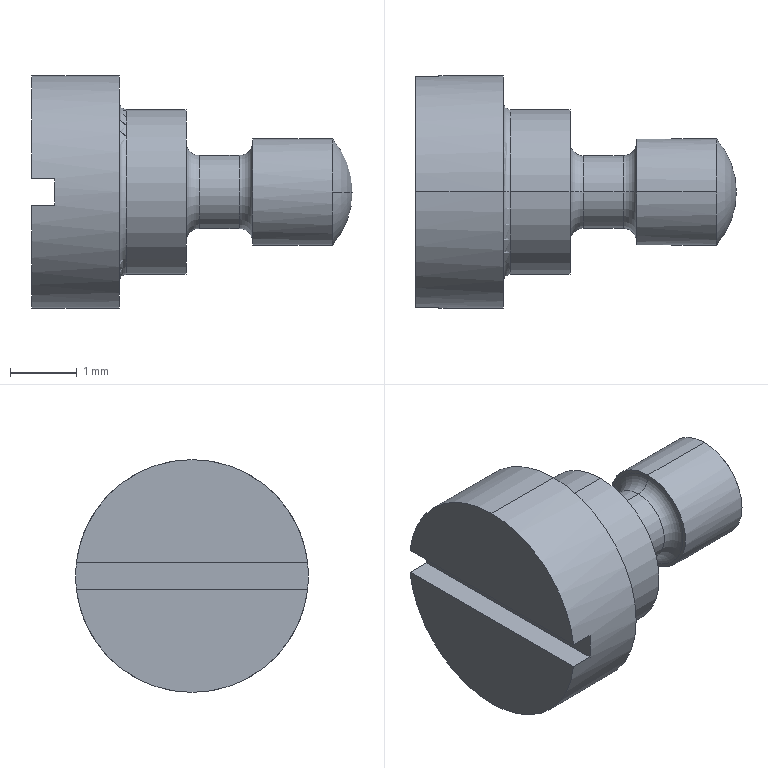Part | STEP file | slotted cheese head screws with shoulder gb_PreviewCfg | 1 solid | 24 faces | box 4.82 x 3.5 x 3.5 mm | volume 20.801 mm3 | cylinder 8 | plane 8 | torus 6 | sphere 2 | commonest cylinder face diameters 1.1 x2 1.6 x2 2.48 x2 3.5 x2